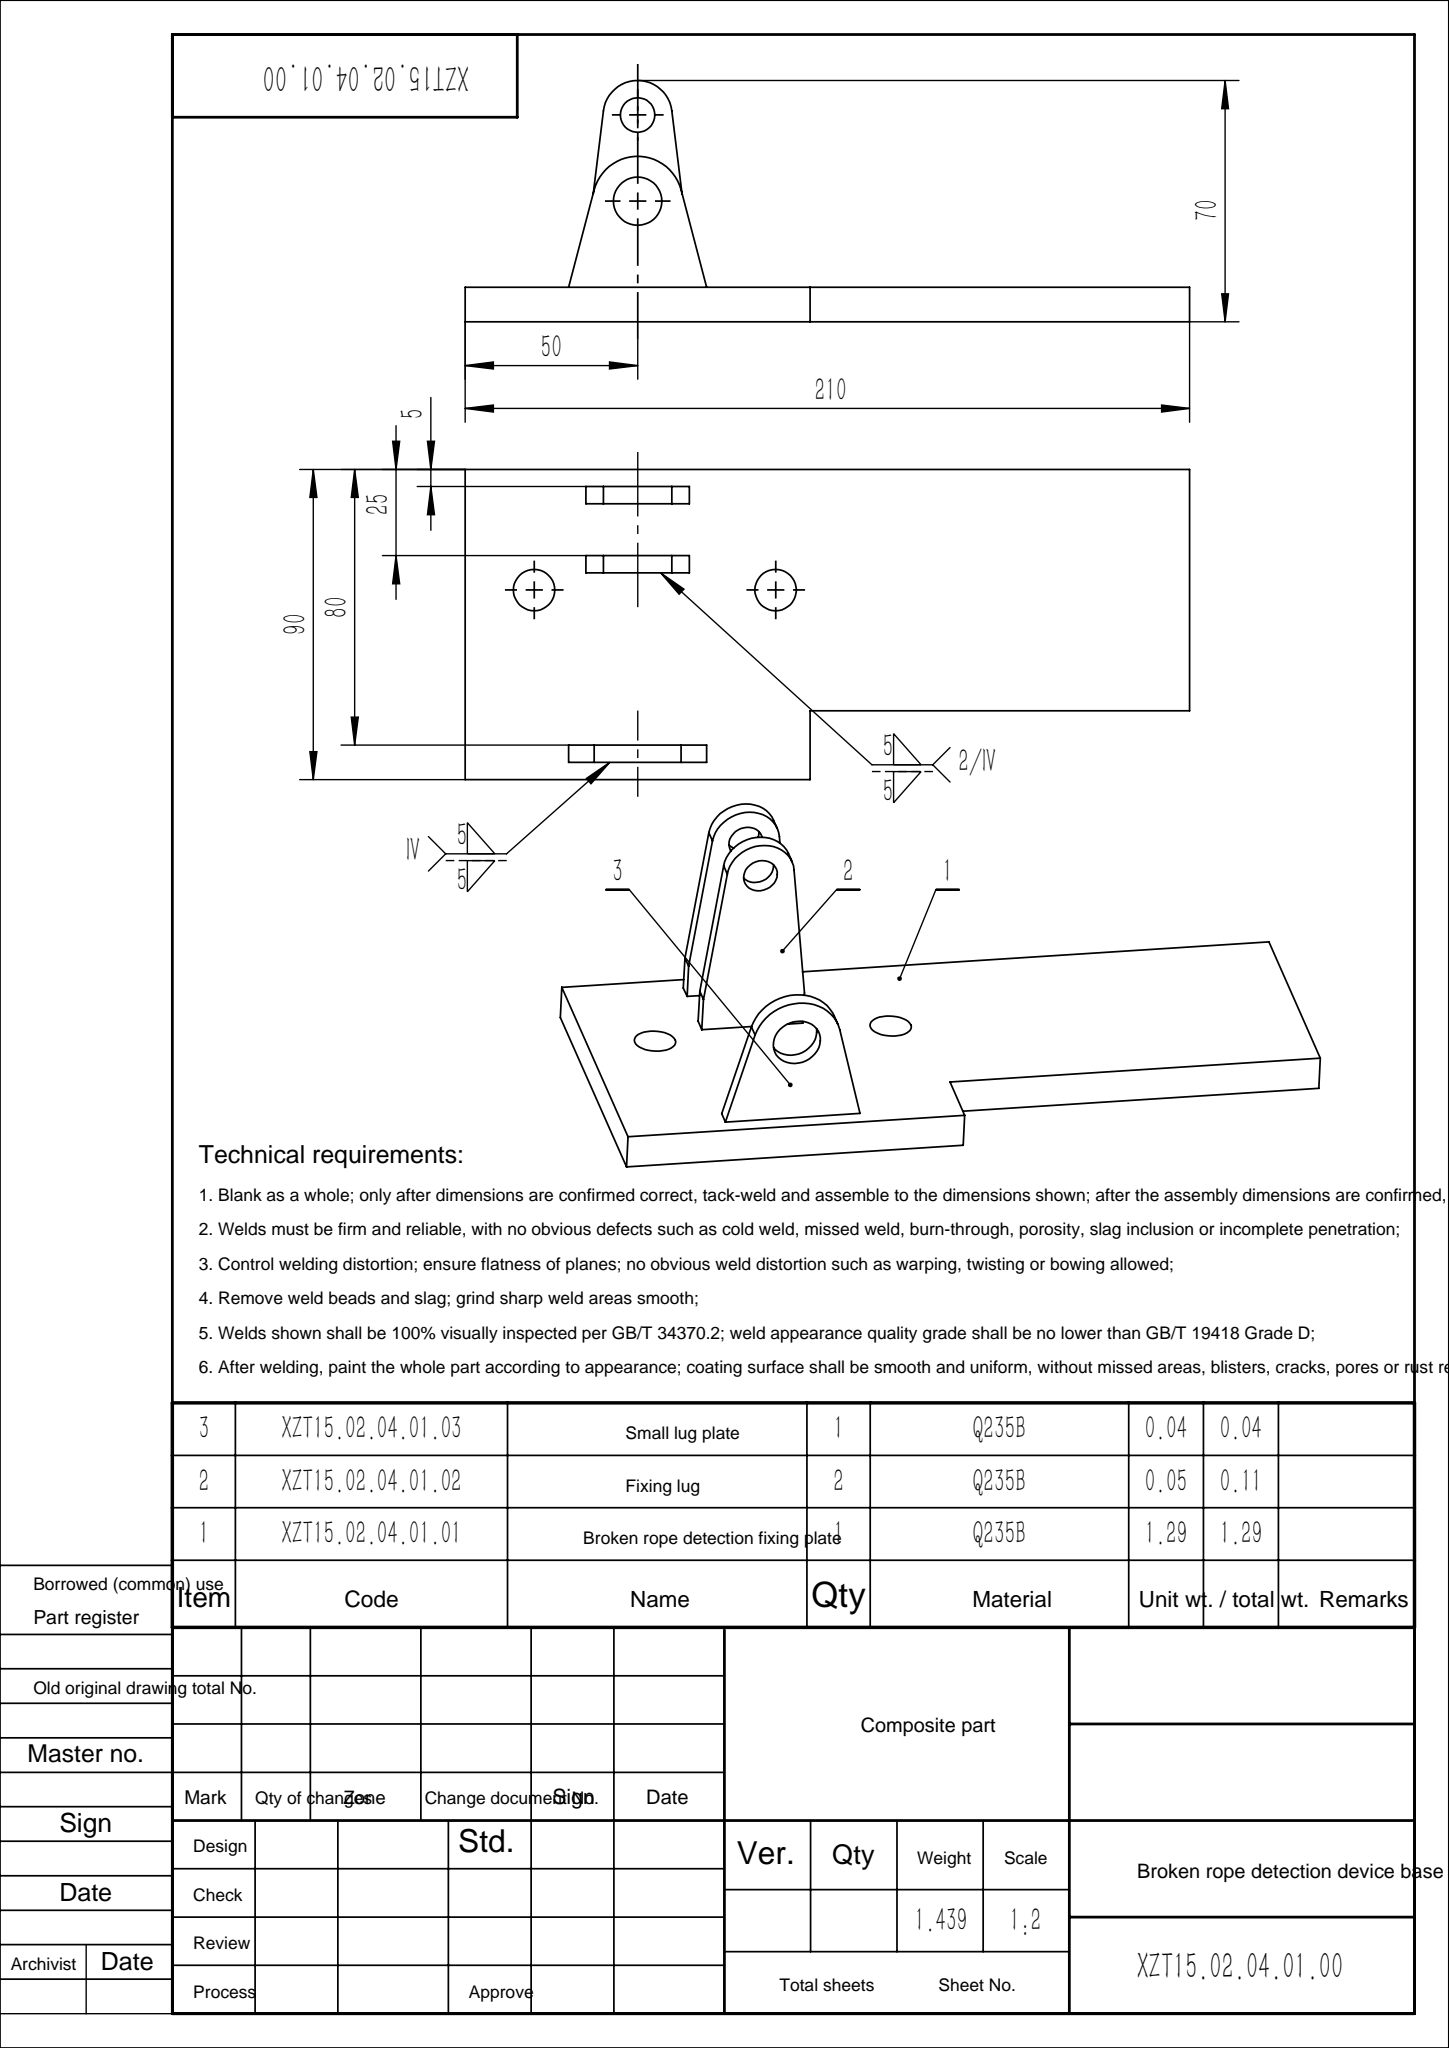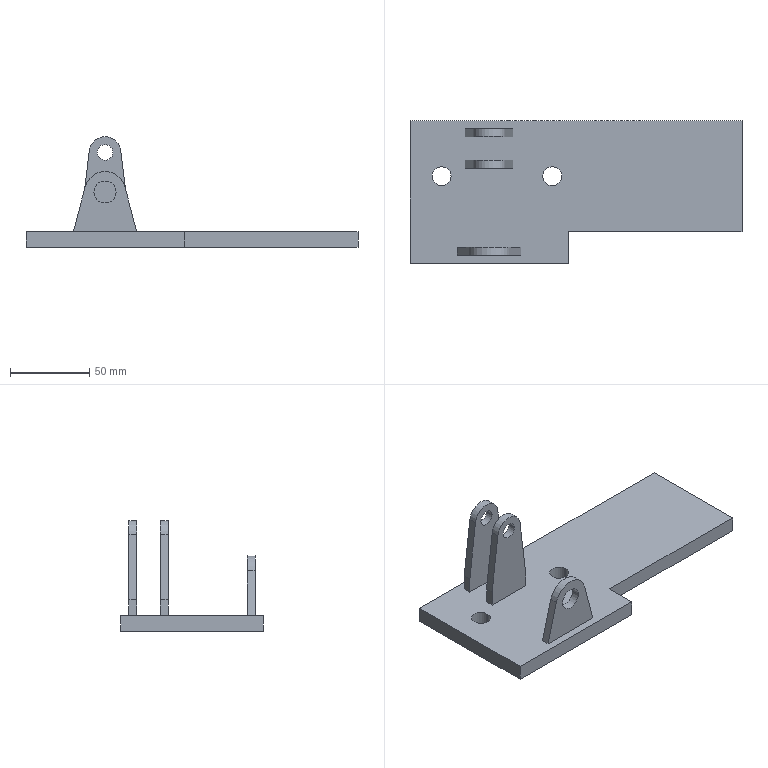Part | SolidWorks | 4 solids | 40 faces | box 210 x 90 x 70 mm | volume 183297 mm3 | plane 27 | cylinder 13 | commonest cylinder face diameters 10 x4 12 x4 14 x2 20 x2 26 x1